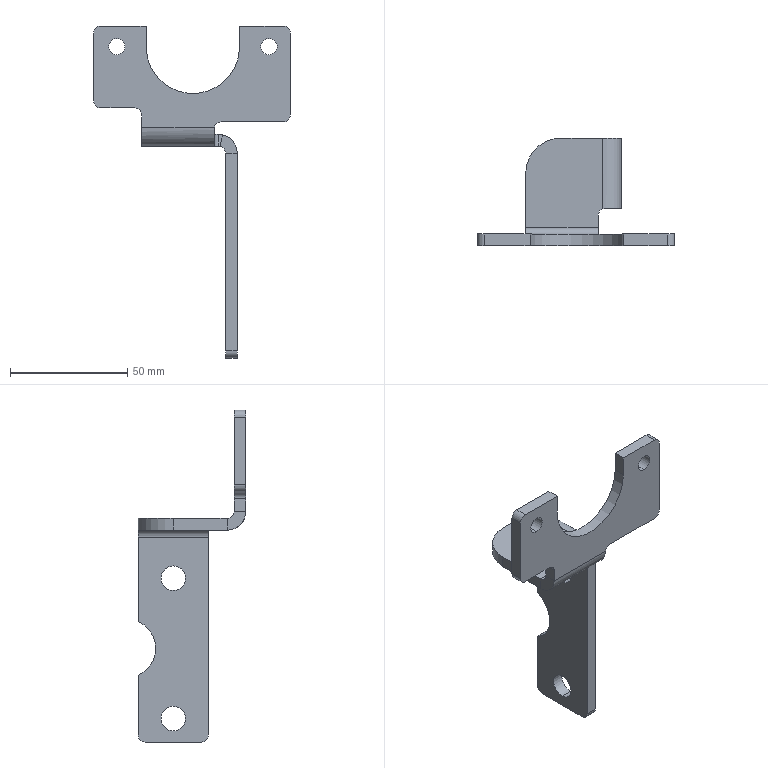Part | SolidWorks | features BaseBody 1 | 1 solid | 52 faces | box 84 x 46 x 141.861 mm | volume 31846 mm3 | plane 26 | cylinder 24 | spline 2 | commonest cylinder face diameters 6 x11 7 x4 10.5 x4 16 x2 25 x1 30 x1